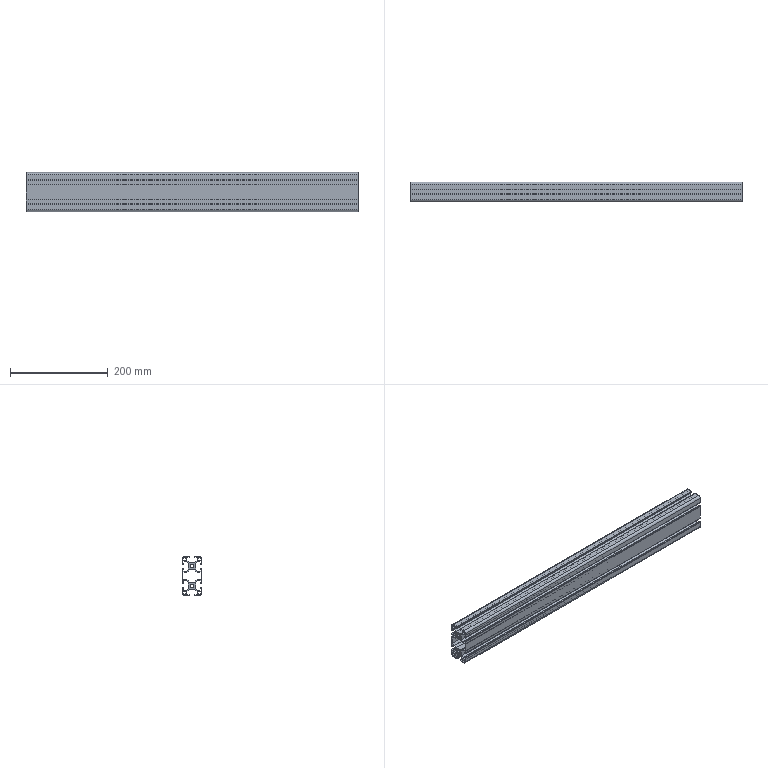Part | 1 solid | 155 faces | box 680 x 40.002 x 80 mm | volume 669387 mm3 | plane 142 | cylinder 13 | commonest cylinder face diameters 9 x5 5 x4 6.8 x4